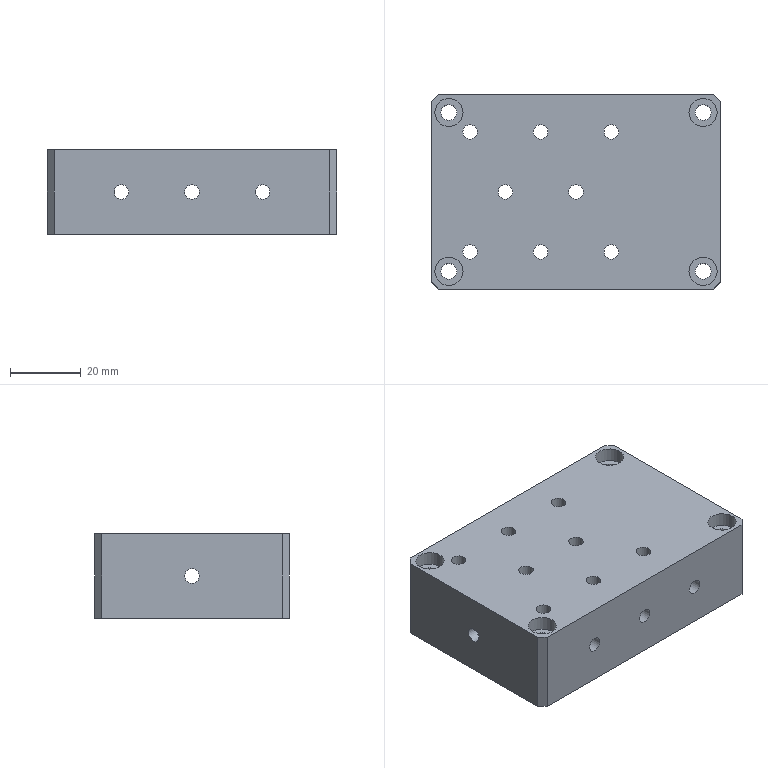NC program | NX | posted with a generic post | part box 82 x 55 x 24 mm
Lines 1 to 72 of 2085:
N10 G17 G21 G94 G90
(FLOOR_WALL , TOOL : D80)
N12 T19 M6
N14 G54
N16 G17 G0 G90 X-86. Y0. B0. C0. S6500 M3
N18 G43 Z30. H19
N20 Z3.
N22 G94 G1 Z0. F1500.
N24 X-83.
N26 X83.
N28 X86.
N30 Z3.
N32 G0 Z30.
N34 M5
(DRILLING , TOOL : D6A45)
N36 T01 M6
N38 G54
N40 G17 G0 G90 X36. Y-22.5 B0. C0. S5000 M3
N42 G43 Z30. H1
N44 G94 G81 G98 Z-1. F350. R3.
N46 X10. Y-17.
N48 X-10.
N50 X-36. Y-22.5
N52 X-30. Y-17.
N54 X-20. Y0.
N56 X-30. Y17.
N58 X-36. Y22.5
N60 X-10. Y17.
N62 X0. Y0.
N64 X10. Y17.
N66 X36. Y22.5
N68 G80
N70 G0 X36. Y22.5 Z30.
N72 M5
(DRILLING_COPY_COPY , TOOL : 4.2ZT)
N74 T04 M6
N76 G54
N78 G17 G0 G90 X10. Y-17. B0. C0. S2000 M3
N80 G43 Z30. H4
N82 G94 G83 G98 Z-9.732 F300. Q2. R3.
N84 X-10.
N86 X0. Y0.
N88 X10. Y17.
N90 X-10.
N92 X-30.
N94 X-20. Y0.
N96 X-30. Y-17.
N98 G80
N100 G0 X-30. Y-17. Z30.
N102 M5
(DRILLING_COPY_COPY_COPY , TOOL : 4.5ZT)
N104 T08 M6
N106 G54
N108 G17 G0 G90 X36. Y22.5 B0. C0. S2000 M3
N110 G43 Z30. H8
N112 G94 G83 G98 Z-26.352 F300. Q2. R3.
N114 Y-22.5
N116 X-36.
N118 Y22.5
N120 G80
N122 G0 X-36. Y22.5 Z30.
N124 M5